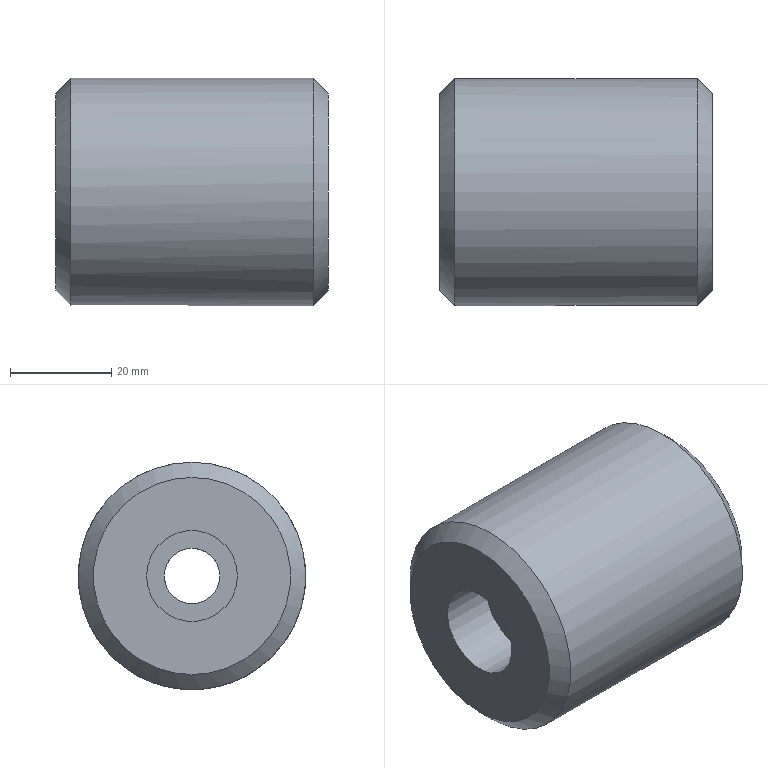Part | STEP file | solid 67 | 1 solid | 8 faces | box 54 x 45 x 45 mm | volume 77782 mm3 | plane 3 | cylinder 3 | cone 2 | commonest cylinder face diameters 11 x1 18 x1 45 x1